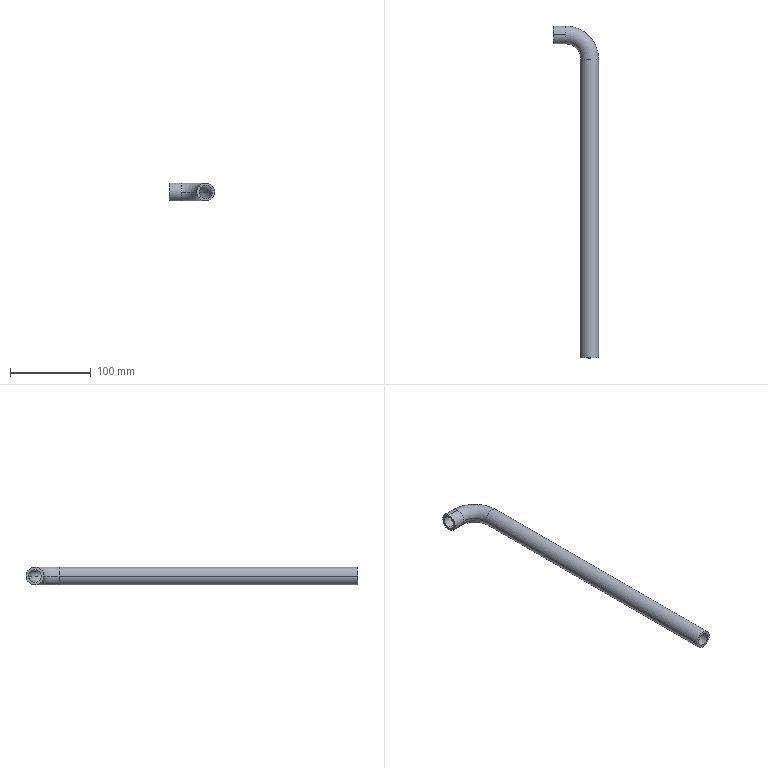Part | SolidWorks | features Sweep 1 | 1 solid | 14 faces | box 56 x 411 x 22 mm | volume 77381 mm3 | cylinder 8 | torus 4 | plane 2 | commonest cylinder face diameters 16 x4 22 x4
STEP:
#1=CARTESIAN_POINT('',(15.,0.,8.));
#2=VERTEX_POINT('',#1);
#3=CARTESIAN_POINT('',(15.,8.,0.));
#4=VERTEX_POINT('',#3);
#5=CARTESIAN_POINT('',(15.,0.,0.));
#6=DIRECTION('',(-1.,0.,0.));
#7=DIRECTION('',(0.,0.,-1.));
#8=AXIS2_PLACEMENT_3D('',#5,#6,#7);
#9=CIRCLE('',#8,8.);
#10=EDGE_CURVE('',#2,#4,#9,.T.);
#11=ORIENTED_EDGE('',*,*,#10,.T.);
#12=CARTESIAN_POINT('',(53.,-30.,0.));
#13=VERTEX_POINT('',#12);
#14=CARTESIAN_POINT('',(15.,-30.,0.));
#15=DIRECTION('',(0.,0.,-1.));
#16=DIRECTION('',(-1.,0.,0.));
#17=AXIS2_PLACEMENT_3D('',#14,#15,#16);
#18=CIRCLE('',#17,38.);
#19=EDGE_CURVE('',#4,#13,#18,.T.);
#20=ORIENTED_EDGE('',*,*,#19,.T.);
#21=CARTESIAN_POINT('',(37.,-30.,0.));
#22=VERTEX_POINT('',#21);
#23=CARTESIAN_POINT('',(45.,-30.,0.));
#24=DIRECTION('',(0.,1.,0.));
#25=DIRECTION('',(0.,0.,-1.));
#26=AXIS2_PLACEMENT_3D('',#23,#24,#25);
#27=CIRCLE('',#26,8.);
#28=EDGE_CURVE('',#22,#13,#27,.T.);
#29=ORIENTED_EDGE('',*,*,#28,.F.);
#30=CARTESIAN_POINT('',(15.,-8.,0.));
#31=VERTEX_POINT('',#30);
#32=CARTESIAN_POINT('',(15.,-30.,0.));
#33=DIRECTION('',(0.,0.,-1.));
#34=DIRECTION('',(-1.,0.,0.));
#35=AXIS2_PLACEMENT_3D('',#32,#33,#34);
#36=CIRCLE('',#35,22.);
#37=EDGE_CURVE('',#31,#22,#36,.T.);
#38=ORIENTED_EDGE('',*,*,#37,.F.);
#39=CARTESIAN_POINT('',(15.,0.,0.));
#40=DIRECTION('',(-1.,0.,0.));
#41=DIRECTION('',(0.,0.,-1.));
#42=AXIS2_PLACEMENT_3D('',#39,#40,#41);
#43=CIRCLE('',#42,8.);
#44=EDGE_CURVE('',#31,#2,#43,.T.);
#45=ORIENTED_EDGE('',*,*,#44,.T.);
#46=EDGE_LOOP('',(#11,#20,#29,#38,#45));
#47=FACE_OUTER_BOUND('',#46,.T.);
#48=CARTESIAN_POINT('',(15.,-30.,0.));
#49=DIRECTION('',(0.,0.,-1.));
#50=DIRECTION('',(-1.,0.,0.));
#51=AXIS2_PLACEMENT_3D('',#48,#49,#50);
#52=TOROIDAL_SURFACE('',#51,30.,8.);
#53=ADVANCED_FACE('',(#47),#52,.F.);
#54=CARTESIAN_POINT('',(15.,0.,-11.));
#55=VERTEX_POINT('',#54);
#56=CARTESIAN_POINT('',(15.,11.,0.));
#57=VERTEX_POINT('',#56);
#58=CARTESIAN_POINT('',(15.,0.,0.));
#59=DIRECTION('',(1.,0.,0.));
#60=DIRECTION('',(0.,0.,-1.));
#61=AXIS2_PLACEMENT_3D('',#58,#59,#60);
#62=CIRCLE('',#61,11.);
#63=EDGE_CURVE('',#55,#57,#62,.T.);
#64=ORIENTED_EDGE('',*,*,#63,.T.);
#65=CARTESIAN_POINT('',(56.,-30.,0.));
#66=VERTEX_POINT('',#65);
#67=CARTESIAN_POINT('',(15.,-30.,0.));
#68=DIRECTION('',(0.,0.,-1.));
#69=DIRECTION('',(-1.,0.,0.));
#70=AXIS2_PLACEMENT_3D('',#67,#68,#69);
#71=CIRCLE('',#70,41.);
#72=EDGE_CURVE('',#57,#66,#71,.T.);
#73=ORIENTED_EDGE('',*,*,#72,.T.);
#74=CARTESIAN_POINT('',(34.,-30.,0.));
#75=VERTEX_POINT('',#74);
#76=CARTESIAN_POINT('',(45.,-30.,0.));
#77=DIRECTION('',(0.,-1.,0.));
#78=DIRECTION('',(0.,0.,-1.));
#79=AXIS2_PLACEMENT_3D('',#76,#77,#78);
#80=CIRCLE('',#79,11.);
#81=EDGE_CURVE('',#75,#66,#80,.T.);
#82=ORIENTED_EDGE('',*,*,#81,.F.);
#83=CARTESIAN_POINT('',(15.,-11.,0.));
#84=VERTEX_POINT('',#83);
#85=CARTESIAN_POINT('',(15.,-30.,0.));
#86=DIRECTION('',(0.,0.,-1.));
#87=DIRECTION('',(-1.,0.,0.));
#88=AXIS2_PLACEMENT_3D('',#85,#86,#87);
#89=CIRCLE('',#88,19.);
#90=EDGE_CURVE('',#84,#75,#89,.T.);
#91=ORIENTED_EDGE('',*,*,#90,.F.);
#92=CARTESIAN_POINT('',(15.,0.,0.));
#93=DIRECTION('',(1.,0.,0.));
#94=DIRECTION('',(0.,0.,-1.));
#95=AXIS2_PLACEMENT_3D('',#92,#93,#94);
#96=CIRCLE('',#95,11.);
#97=EDGE_CURVE('',#84,#55,#96,.T.);
#98=ORIENTED_EDGE('',*,*,#97,.T.);
#99=EDGE_LOOP('',(#64,#73,#82,#91,#98));
#100=FACE_OUTER_BOUND('',#99,.T.);
#101=CARTESIAN_POINT('',(15.,-30.,0.));
#102=DIRECTION('',(0.,0.,-1.));
#103=DIRECTION('',(-1.,0.,0.));
#104=AXIS2_PLACEMENT_3D('',#101,#102,#103);
#105=TOROIDAL_SURFACE('',#104,30.,11.);
#106=ADVANCED_FACE('',(#100),#105,.T.);
#107=CARTESIAN_POINT('',(45.,-30.,0.));
#108=DIRECTION('',(0.,1.,0.));
#109=DIRECTION('',(0.,0.,-1.));
#110=AXIS2_PLACEMENT_3D('',#107,#108,#109);
#111=CIRCLE('',#110,8.);
#112=EDGE_CURVE('',#13,#22,#111,.T.);
#113=ORIENTED_EDGE('',*,*,#112,.T.);
#114=CARTESIAN_POINT('',(37.,-400.,0.));
#115=VERTEX_POINT('',#114);
#116=CARTESIAN_POINT('',(37.,-30.,0.));
#117=DIRECTION('',(0.,-1.,0.));
#118=VECTOR('',#117,1000.);
#119=LINE('',#116,#118);
#120=EDGE_CURVE('',#22,#115,#119,.T.);
#121=ORIENTED_EDGE('',*,*,#120,.T.);
#122=CARTESIAN_POINT('',(53.,-400.,0.));
#123=VERTEX_POINT('',#122);
#124=CARTESIAN_POINT('',(45.,-400.,0.));
#125=DIRECTION('',(0.,1.,0.));
#126=DIRECTION('',(0.,0.,-1.));
#127=AXIS2_PLACEMENT_3D('',#124,#125,#126);
#128=CIRCLE('',#127,8.);
#129=EDGE_CURVE('',#123,#115,#128,.T.);
#130=ORIENTED_EDGE('',*,*,#129,.F.);
#131=CARTESIAN_POINT('',(53.,-30.,0.));
#132=DIRECTION('',(0.,-1.,0.));
#133=VECTOR('',#132,1000.);
#134=LINE('',#131,#133);
#135=EDGE_CURVE('',#13,#123,#134,.T.);
#136=ORIENTED_EDGE('',*,*,#135,.F.);
#137=EDGE_LOOP('',(#113,#121,#130,#136));
#138=FACE_OUTER_BOUND('',#137,.T.);
#139=CARTESIAN_POINT('',(45.,-30.,0.));
#140=DIRECTION('',(0.,-1.,0.));
#141=DIRECTION('',(1.,0.,0.));
#142=AXIS2_PLACEMENT_3D('',#139,#140,#141);
#143=CYLINDRICAL_SURFACE('',#142,8.);
#144=ADVANCED_FACE('',(#138),#143,.F.);
#145=CARTESIAN_POINT('',(0.,0.,-8.));
#146=VERTEX_POINT('',#145);
#147=CARTESIAN_POINT('',(0.,0.,8.));
#148=VERTEX_POINT('',#147);
#149=CARTESIAN_POINT('',(0.,0.,0.));
#150=DIRECTION('',(-1.,0.,0.));
#151=DIRECTION('',(0.,0.,-1.));
#152=AXIS2_PLACEMENT_3D('',#149,#150,#151);
#153=CIRCLE('',#152,8.);
#154=EDGE_CURVE('',#146,#148,#153,.T.);
#155=ORIENTED_EDGE('',*,*,#154,.T.);
#156=CARTESIAN_POINT('',(0.,0.,8.));
#157=DIRECTION('',(1.,0.,0.));
#158=VECTOR('',#157,1000.);
#159=LINE('',#156,#158);
#160=EDGE_CURVE('',#148,#2,#159,.T.);
#161=ORIENTED_EDGE('',*,*,#160,.T.);
#162=ORIENTED_EDGE('',*,*,#44,.F.);
#163=CARTESIAN_POINT('',(15.,0.,-8.));
#164=VERTEX_POINT('',#163);
#165=CARTESIAN_POINT('',(15.,0.,0.));
#166=DIRECTION('',(-1.,0.,0.));
#167=DIRECTION('',(0.,0.,-1.));
#168=AXIS2_PLACEMENT_3D('',#165,#166,#167);
#169=CIRCLE('',#168,8.);
#170=EDGE_CURVE('',#164,#31,#169,.T.);
#171=ORIENTED_EDGE('',*,*,#170,.F.);
#172=CARTESIAN_POINT('',(0.,0.,-8.));
#173=DIRECTION('',(1.,0.,0.));
#174=VECTOR('',#173,1000.);
#175=LINE('',#172,#174);
#176=EDGE_CURVE('',#146,#164,#175,.T.);
#177=ORIENTED_EDGE('',*,*,#176,.F.);
#178=EDGE_LOOP('',(#155,#161,#162,#171,#177));
#179=FACE_OUTER_BOUND('',#178,.T.);
#180=CARTESIAN_POINT('',(0.,0.,0.));
#181=DIRECTION('',(1.,0.,0.));
#182=DIRECTION('',(0.,0.,-1.));
#183=AXIS2_PLACEMENT_3D('',#180,#181,#182);
#184=CYLINDRICAL_SURFACE('',#183,8.);
#185=ADVANCED_FACE('',(#179),#184,.F.);
#186=CARTESIAN_POINT('',(45.,-30.,0.));
#187=DIRECTION('',(0.,-1.,0.));
#188=DIRECTION('',(0.,0.,-1.));
#189=AXIS2_PLACEMENT_3D('',#186,#187,#188);
#190=CIRCLE('',#189,11.);
#191=EDGE_CURVE('',#66,#75,#190,.T.);
#192=ORIENTED_EDGE('',*,*,#191,.T.);
#193=CARTESIAN_POINT('',(34.,-400.,0.));
#194=VERTEX_POINT('',#193);
#195=CARTESIAN_POINT('',(34.,-30.,0.));
#196=DIRECTION('',(0.,-1.,0.));
#197=VECTOR('',#196,1000.);
#198=LINE('',#195,#197);
#199=EDGE_CURVE('',#75,#194,#198,.T.);
#200=ORIENTED_EDGE('',*,*,#199,.T.);
#201=CARTESIAN_POINT('',(56.,-400.,0.));
#202=VERTEX_POINT('',#201);
#203=CARTESIAN_POINT('',(45.,-400.,0.));
#204=DIRECTION('',(0.,-1.,0.));
#205=DIRECTION('',(0.,0.,-1.));
#206=AXIS2_PLACEMENT_3D('',#203,#204,#205);
#207=CIRCLE('',#206,11.);
#208=EDGE_CURVE('',#202,#194,#207,.T.);
#209=ORIENTED_EDGE('',*,*,#208,.F.);
#210=CARTESIAN_POINT('',(56.,-30.,0.));
#211=DIRECTION('',(0.,-1.,0.));
#212=VECTOR('',#211,1000.);
#213=LINE('',#210,#212);
#214=EDGE_CURVE('',#66,#202,#213,.T.);
#215=ORIENTED_EDGE('',*,*,#214,.F.);
#216=EDGE_LOOP('',(#192,#200,#209,#215));
#217=FACE_OUTER_BOUND('',#216,.T.);
#218=CARTESIAN_POINT('',(45.,-30.,0.));
#219=DIRECTION('',(0.,-1.,0.));
#220=DIRECTION('',(1.,0.,0.));
#221=AXIS2_PLACEMENT_3D('',#218,#219,#220);
#222=CYLINDRICAL_SURFACE('',#221,11.);
#223=ADVANCED_FACE('',(#217),#222,.T.);
#224=CARTESIAN_POINT('',(0.,0.,-11.));
#225=VERTEX_POINT('',#224);
#226=CARTESIAN_POINT('',(0.,0.,11.));
#227=VERTEX_POINT('',#226);
#228=CARTESIAN_POINT('',(0.,0.,0.));
#229=DIRECTION('',(1.,0.,0.));
#230=DIRECTION('',(0.,0.,-1.));
#231=AXIS2_PLACEMENT_3D('',#228,#229,#230);
#232=CIRCLE('',#231,11.);
#233=EDGE_CURVE('',#225,#227,#232,.T.);
#234=ORIENTED_EDGE('',*,*,#233,.T.);
#235=CARTESIAN_POINT('',(15.,0.,11.));
#236=VERTEX_POINT('',#235);
#237=CARTESIAN_POINT('',(0.,0.,11.));
#238=DIRECTION('',(1.,0.,0.));
#239=VECTOR('',#238,1000.);
#240=LINE('',#237,#239);
#241=EDGE_CURVE('',#227,#236,#240,.T.);
#242=ORIENTED_EDGE('',*,*,#241,.T.);
#243=CARTESIAN_POINT('',(15.,0.,0.));
#244=DIRECTION('',(1.,0.,0.));
#245=DIRECTION('',(0.,0.,-1.));
#246=AXIS2_PLACEMENT_3D('',#243,#244,#245);
#247=CIRCLE('',#246,11.);
#248=EDGE_CURVE('',#57,#236,#247,.T.);
#249=ORIENTED_EDGE('',*,*,#248,.F.);
#250=ORIENTED_EDGE('',*,*,#63,.F.);
#251=CARTESIAN_POINT('',(0.,0.,-11.));
#252=DIRECTION('',(1.,0.,0.));
#253=VECTOR('',#252,1000.);
#254=LINE('',#251,#253);
#255=EDGE_CURVE('',#225,#55,#254,.T.);
#256=ORIENTED_EDGE('',*,*,#255,.F.);
#257=EDGE_LOOP('',(#234,#242,#249,#250,#256));
#258=FACE_OUTER_BOUND('',#257,.T.);
#259=CARTESIAN_POINT('',(0.,0.,0.));
#260=DIRECTION('',(1.,0.,0.));
#261=DIRECTION('',(0.,0.,-1.));
#262=AXIS2_PLACEMENT_3D('',#259,#260,#261);
#263=CYLINDRICAL_SURFACE('',#262,11.);
#264=ADVANCED_FACE('',(#258),#263,.T.);
#265=ORIENTED_EDGE('',*,*,#120,.F.);
#266=ORIENTED_EDGE('',*,*,#28,.T.);
#267=ORIENTED_EDGE('',*,*,#135,.T.);
#268=CARTESIAN_POINT('',(45.,-400.,0.));
#269=DIRECTION('',(0.,1.,0.));
#270=DIRECTION('',(0.,0.,-1.));
#271=AXIS2_PLACEMENT_3D('',#268,#269,#270);
#272=CIRCLE('',#271,8.);
#273=EDGE_CURVE('',#115,#123,#272,.T.);
#274=ORIENTED_EDGE('',*,*,#273,.F.);
#275=EDGE_LOOP('',(#265,#266,#267,#274));
#276=FACE_OUTER_BOUND('',#275,.T.);
#277=CARTESIAN_POINT('',(45.,-30.,0.));
#278=DIRECTION('',(0.,-1.,0.));
#279=DIRECTION('',(1.,0.,0.));
#280=AXIS2_PLACEMENT_3D('',#277,#278,#279);
#281=CYLINDRICAL_SURFACE('',#280,8.);
#282=ADVANCED_FACE('',(#276),#281,.F.);
#283=ORIENTED_EDGE('',*,*,#19,.F.);
#284=CARTESIAN_POINT('',(15.,0.,0.));
#285=DIRECTION('',(-1.,0.,0.));
#286=DIRECTION('',(0.,0.,-1.));
#287=AXIS2_PLACEMENT_3D('',#284,#285,#286);
#288=CIRCLE('',#287,8.);
#289=EDGE_CURVE('',#4,#164,#288,.T.);
#290=ORIENTED_EDGE('',*,*,#289,.T.);
#291=ORIENTED_EDGE('',*,*,#170,.T.);
#292=ORIENTED_EDGE('',*,*,#37,.T.);
#293=ORIENTED_EDGE('',*,*,#112,.F.);
#294=EDGE_LOOP('',(#283,#290,#291,#292,#293));
#295=FACE_OUTER_BOUND('',#294,.T.);
#296=CARTESIAN_POINT('',(15.,-30.,0.));
#297=DIRECTION('',(0.,0.,-1.));
#298=DIRECTION('',(-1.,0.,0.));
#299=AXIS2_PLACEMENT_3D('',#296,#297,#298);
#300=TOROIDAL_SURFACE('',#299,30.,8.);
#301=ADVANCED_FACE('',(#295),#300,.F.);
#302=ORIENTED_EDGE('',*,*,#160,.F.);
#303=CARTESIAN_POINT('',(0.,0.,0.));
#304=DIRECTION('',(-1.,0.,0.));
#305=DIRECTION('',(0.,0.,-1.));
#306=AXIS2_PLACEMENT_3D('',#303,#304,#305);
#307=CIRCLE('',#306,8.);
#308=EDGE_CURVE('',#148,#146,#307,.T.);
#309=ORIENTED_EDGE('',*,*,#308,.T.);
#310=ORIENTED_EDGE('',*,*,#176,.T.);
#311=ORIENTED_EDGE('',*,*,#289,.F.);
#312=ORIENTED_EDGE('',*,*,#10,.F.);
#313=EDGE_LOOP('',(#302,#309,#310,#311,#312));
#314=FACE_OUTER_BOUND('',#313,.T.);
#315=CARTESIAN_POINT('',(0.,0.,0.));
#316=DIRECTION('',(1.,0.,0.));
#317=DIRECTION('',(0.,0.,-1.));
#318=AXIS2_PLACEMENT_3D('',#315,#316,#317);
#319=CYLINDRICAL_SURFACE('',#318,8.);
#320=ADVANCED_FACE('',(#314),#319,.F.);
#321=ORIENTED_EDGE('',*,*,#129,.T.);
#322=ORIENTED_EDGE('',*,*,#273,.T.);
#323=EDGE_LOOP('',(#321,#322));
#324=FACE_BOUND('',#323,.T.);
#325=ORIENTED_EDGE('',*,*,#208,.T.);
#326=CARTESIAN_POINT('',(45.,-400.,0.));
#327=DIRECTION('',(0.,-1.,0.));
#328=DIRECTION('',(0.,0.,-1.));
#329=AXIS2_PLACEMENT_3D('',#326,#327,#328);
#330=CIRCLE('',#329,11.);
#331=EDGE_CURVE('',#194,#202,#330,.T.);
#332=ORIENTED_EDGE('',*,*,#331,.T.);
#333=EDGE_LOOP('',(#325,#332));
#334=FACE_OUTER_BOUND('',#333,.T.);
#335=CARTESIAN_POINT('',(45.,-400.,0.));
#336=DIRECTION('',(0.,-1.,0.));
#337=DIRECTION('',(0.,0.,-1.));
#338=AXIS2_PLACEMENT_3D('',#335,#336,#337);
#339=PLANE('',#338);
#340=ADVANCED_FACE('',(#324,#334),#339,.T.);
#341=ORIENTED_EDGE('',*,*,#154,.F.);
#342=ORIENTED_EDGE('',*,*,#308,.F.);
#343=EDGE_LOOP('',(#341,#342));
#344=FACE_BOUND('',#343,.T.);
#345=ORIENTED_EDGE('',*,*,#233,.F.);
#346=CARTESIAN_POINT('',(0.,0.,0.));
#347=DIRECTION('',(1.,0.,0.));
#348=DIRECTION('',(0.,0.,-1.));
#349=AXIS2_PLACEMENT_3D('',#346,#347,#348);
#350=CIRCLE('',#349,11.);
#351=EDGE_CURVE('',#227,#225,#350,.T.);
#352=ORIENTED_EDGE('',*,*,#351,.F.);
#353=EDGE_LOOP('',(#345,#352));
#354=FACE_OUTER_BOUND('',#353,.T.);
#355=CARTESIAN_POINT('',(0.,0.,0.));
#356=DIRECTION('',(1.,0.,0.));
#357=DIRECTION('',(0.,0.,-1.));
#358=AXIS2_PLACEMENT_3D('',#355,#356,#357);
#359=PLANE('',#358);
#360=ADVANCED_FACE('',(#344,#354),#359,.F.);
#361=ORIENTED_EDGE('',*,*,#199,.F.);
#362=ORIENTED_EDGE('',*,*,#81,.T.);
#363=ORIENTED_EDGE('',*,*,#214,.T.);
#364=ORIENTED_EDGE('',*,*,#331,.F.);
#365=EDGE_LOOP('',(#361,#362,#363,#364));
#366=FACE_OUTER_BOUND('',#365,.T.);
#367=CARTESIAN_POINT('',(45.,-30.,0.));
#368=DIRECTION('',(0.,-1.,0.));
#369=DIRECTION('',(1.,0.,0.));
#370=AXIS2_PLACEMENT_3D('',#367,#368,#369);
#371=CYLINDRICAL_SURFACE('',#370,11.);
#372=ADVANCED_FACE('',(#366),#371,.T.);
#373=ORIENTED_EDGE('',*,*,#72,.F.);
#374=ORIENTED_EDGE('',*,*,#248,.T.);
#375=CARTESIAN_POINT('',(15.,0.,0.));
#376=DIRECTION('',(1.,0.,0.));
#377=DIRECTION('',(0.,0.,-1.));
#378=AXIS2_PLACEMENT_3D('',#375,#376,#377);
#379=CIRCLE('',#378,11.);
#380=EDGE_CURVE('',#236,#84,#379,.T.);
#381=ORIENTED_EDGE('',*,*,#380,.T.);
#382=ORIENTED_EDGE('',*,*,#90,.T.);
#383=ORIENTED_EDGE('',*,*,#191,.F.);
#384=EDGE_LOOP('',(#373,#374,#381,#382,#383));
#385=FACE_OUTER_BOUND('',#384,.T.);
#386=CARTESIAN_POINT('',(15.,-30.,0.));
#387=DIRECTION('',(0.,0.,-1.));
#388=DIRECTION('',(-1.,0.,0.));
#389=AXIS2_PLACEMENT_3D('',#386,#387,#388);
#390=TOROIDAL_SURFACE('',#389,30.,11.);
#391=ADVANCED_FACE('',(#385),#390,.T.);
#392=ORIENTED_EDGE('',*,*,#241,.F.);
#393=ORIENTED_EDGE('',*,*,#351,.T.);
#394=ORIENTED_EDGE('',*,*,#255,.T.);
#395=ORIENTED_EDGE('',*,*,#97,.F.);
#396=ORIENTED_EDGE('',*,*,#380,.F.);
#397=EDGE_LOOP('',(#392,#393,#394,#395,#396));
#398=FACE_OUTER_BOUND('',#397,.T.);
#399=CARTESIAN_POINT('',(0.,0.,0.));
#400=DIRECTION('',(1.,0.,0.));
#401=DIRECTION('',(0.,0.,-1.));
#402=AXIS2_PLACEMENT_3D('',#399,#400,#401);
#403=CYLINDRICAL_SURFACE('',#402,11.);
#404=ADVANCED_FACE('',(#398),#403,.T.);
#405=CLOSED_SHELL('',(#53,#106,#144,#185,#223,#264,#282,#301,#320,#340,#360,#372,#391,#404));
#406=MANIFOLD_SOLID_BREP('',#405);
#407=CARTESIAN_POINT('',(0.,0.,0.));
#408=DIRECTION('',(0.,0.,1.));
#409=DIRECTION('',(1.,0.,0.));
#410=AXIS2_PLACEMENT_3D('',#407,#408,#409);
#411=(LENGTH_UNIT()NAMED_UNIT(*)SI_UNIT(.MILLI.,.METRE.));
#412=UNCERTAINTY_MEASURE_WITH_UNIT(LENGTH_MEASURE(0.00001),#411,'','');
#413=(NAMED_UNIT(*)PLANE_ANGLE_UNIT()SI_UNIT($,.RADIAN.));
#414=(NAMED_UNIT(*)SI_UNIT($,.STERADIAN.)SOLID_ANGLE_UNIT());
#415=(GEOMETRIC_REPRESENTATION_CONTEXT(3)GLOBAL_UNCERTAINTY_ASSIGNED_CONTEXT((#412))GLOBAL_UNIT_ASSIGNED_CONTEXT((#411,#413,#414))REPRESENTATION_CONTEXT('',''));
#416=ADVANCED_BREP_SHAPE_REPRESENTATION('',(#406,#410),#415);